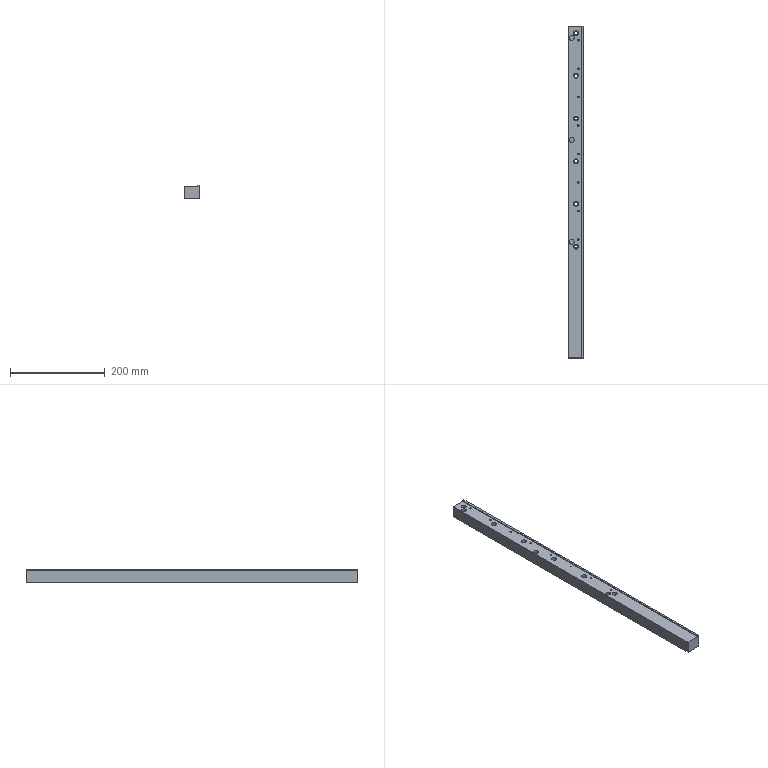Part | STEP file | ASND-0110-LPMF01-029 | 1 solid | 79 faces | box 32 x 700 x 28 mm | volume 574671 mm3 | cylinder 46 | plane 17 | cone 16 | commonest cylinder face diameters 3.3 x16 6.5 x12 10.5 x12 10 x6